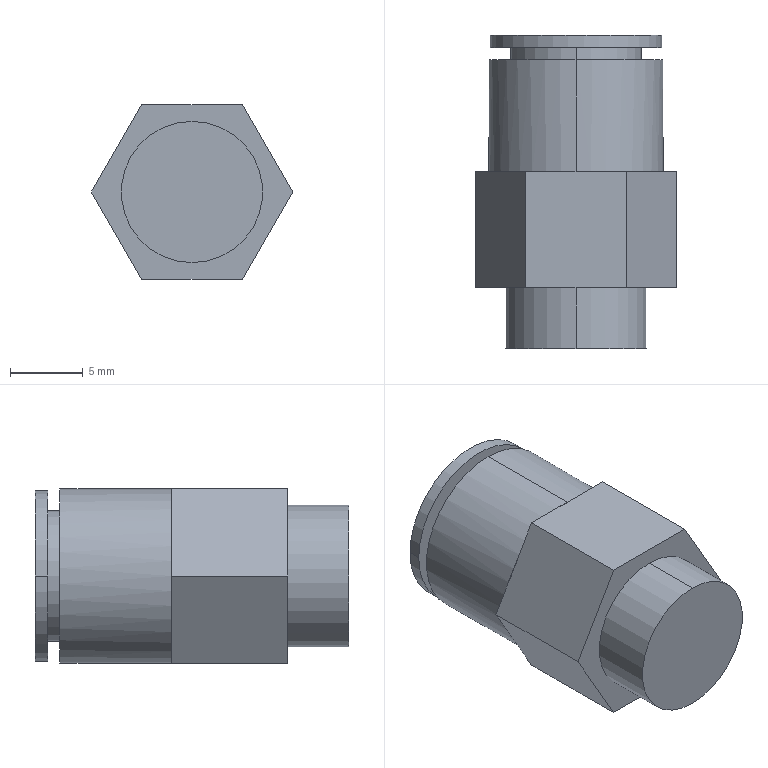Part | SolidWorks | features BaseBody 1 | 1 solid | 28 faces | box 13.856 x 21.6 x 12 mm | volume 1847 mm3 | plane 18 | cylinder 10 | commonest cylinder face diameters 6 x2 9 x2 9.728 x2 11.8 x2 12 x2
STEP:
#1=CARTESIAN_POINT('',(0.,1.5,3.));
#2=VERTEX_POINT('',#1);
#3=CARTESIAN_POINT('',(0.,1.5,-3.));
#4=VERTEX_POINT('',#3);
#5=CARTESIAN_POINT('',(0.,1.5,0.));
#6=DIRECTION('',(0.,-1.,0.));
#7=DIRECTION('',(0.,0.,1.));
#8=AXIS2_PLACEMENT_3D('',#5,#6,#7);
#9=CIRCLE('',#8,3.);
#10=EDGE_CURVE('',#2,#4,#9,.T.);
#11=ORIENTED_EDGE('',*,*,#10,.T.);
#12=CARTESIAN_POINT('',(0.,18.5,-3.));
#13=VERTEX_POINT('',#12);
#14=CARTESIAN_POINT('',(0.,1.5,-3.));
#15=DIRECTION('',(0.,1.,0.));
#16=VECTOR('',#15,1000.);
#17=LINE('',#14,#16);
#18=EDGE_CURVE('',#4,#13,#17,.T.);
#19=ORIENTED_EDGE('',*,*,#18,.T.);
#20=CARTESIAN_POINT('',(0.,18.5,3.));
#21=VERTEX_POINT('',#20);
#22=CARTESIAN_POINT('',(0.,18.5,0.));
#23=DIRECTION('',(0.,1.,0.));
#24=DIRECTION('',(0.,0.,1.));
#25=AXIS2_PLACEMENT_3D('',#22,#23,#24);
#26=CIRCLE('',#25,3.);
#27=EDGE_CURVE('',#13,#21,#26,.T.);
#28=ORIENTED_EDGE('',*,*,#27,.T.);
#29=CARTESIAN_POINT('',(0.,1.5,3.));
#30=DIRECTION('',(0.,1.,0.));
#31=VECTOR('',#30,1000.);
#32=LINE('',#29,#31);
#33=EDGE_CURVE('',#2,#21,#32,.T.);
#34=ORIENTED_EDGE('',*,*,#33,.F.);
#35=EDGE_LOOP('',(#11,#19,#28,#34));
#36=FACE_OUTER_BOUND('',#35,.T.);
#37=CARTESIAN_POINT('',(0.,1.5,0.));
#38=DIRECTION('',(0.,1.,0.));
#39=DIRECTION('',(0.,0.,1.));
#40=AXIS2_PLACEMENT_3D('',#37,#38,#39);
#41=CYLINDRICAL_SURFACE('',#40,3.);
#42=ADVANCED_FACE('',(#36),#41,.F.);
#43=CARTESIAN_POINT('',(-5.9,17.65,0.));
#44=VERTEX_POINT('',#43);
#45=CARTESIAN_POINT('',(5.9,17.65,0.));
#46=VERTEX_POINT('',#45);
#47=CARTESIAN_POINT('',(0.,17.65,0.));
#48=DIRECTION('',(0.,1.,0.));
#49=DIRECTION('',(-1.,0.,0.));
#50=AXIS2_PLACEMENT_3D('',#47,#48,#49);
#51=CIRCLE('',#50,5.9);
#52=EDGE_CURVE('',#44,#46,#51,.T.);
#53=ORIENTED_EDGE('',*,*,#52,.T.);
#54=CARTESIAN_POINT('',(5.9,18.5,0.));
#55=VERTEX_POINT('',#54);
#56=CARTESIAN_POINT('',(5.9,18.5,0.));
#57=DIRECTION('',(0.,1.,0.));
#58=VECTOR('',#57,1000.);
#59=LINE('',#56,#58);
#60=EDGE_CURVE('',#46,#55,#59,.T.);
#61=ORIENTED_EDGE('',*,*,#60,.T.);
#62=CARTESIAN_POINT('',(-5.9,18.5,0.));
#63=VERTEX_POINT('',#62);
#64=CARTESIAN_POINT('',(0.,18.5,0.));
#65=DIRECTION('',(0.,1.,0.));
#66=DIRECTION('',(-1.,0.,0.));
#67=AXIS2_PLACEMENT_3D('',#64,#65,#66);
#68=CIRCLE('',#67,5.9);
#69=EDGE_CURVE('',#63,#55,#68,.T.);
#70=ORIENTED_EDGE('',*,*,#69,.F.);
#71=CARTESIAN_POINT('',(-5.9,18.5,0.));
#72=DIRECTION('',(0.,1.,0.));
#73=VECTOR('',#72,1000.);
#74=LINE('',#71,#73);
#75=EDGE_CURVE('',#44,#63,#74,.T.);
#76=ORIENTED_EDGE('',*,*,#75,.F.);
#77=EDGE_LOOP('',(#53,#61,#70,#76));
#78=FACE_OUTER_BOUND('',#77,.T.);
#79=CARTESIAN_POINT('',(0.,18.5,0.));
#80=DIRECTION('',(0.,1.,0.));
#81=DIRECTION('',(-1.,0.,0.));
#82=AXIS2_PLACEMENT_3D('',#79,#80,#81);
#83=CYLINDRICAL_SURFACE('',#82,5.9);
#84=ADVANCED_FACE('',(#78),#83,.T.);
#85=CARTESIAN_POINT('',(0.,16.8,4.5));
#86=VERTEX_POINT('',#85);
#87=CARTESIAN_POINT('',(0.,16.8,-4.5));
#88=VERTEX_POINT('',#87);
#89=CARTESIAN_POINT('',(0.,16.8,0.));
#90=DIRECTION('',(0.,1.,0.));
#91=DIRECTION('',(0.,0.,1.));
#92=AXIS2_PLACEMENT_3D('',#89,#90,#91);
#93=CIRCLE('',#92,4.5);
#94=EDGE_CURVE('',#86,#88,#93,.T.);
#95=ORIENTED_EDGE('',*,*,#94,.T.);
#96=CARTESIAN_POINT('',(0.,17.65,-4.5));
#97=VERTEX_POINT('',#96);
#98=CARTESIAN_POINT('',(0.,17.65,-4.5));
#99=DIRECTION('',(0.,1.,0.));
#100=VECTOR('',#99,1000.);
#101=LINE('',#98,#100);
#102=EDGE_CURVE('',#88,#97,#101,.T.);
#103=ORIENTED_EDGE('',*,*,#102,.T.);
#104=CARTESIAN_POINT('',(0.,17.65,4.5));
#105=VERTEX_POINT('',#104);
#106=CARTESIAN_POINT('',(0.,17.65,0.));
#107=DIRECTION('',(0.,1.,0.));
#108=DIRECTION('',(0.,0.,1.));
#109=AXIS2_PLACEMENT_3D('',#106,#107,#108);
#110=CIRCLE('',#109,4.5);
#111=EDGE_CURVE('',#105,#97,#110,.T.);
#112=ORIENTED_EDGE('',*,*,#111,.F.);
#113=CARTESIAN_POINT('',(0.,17.65,4.5));
#114=DIRECTION('',(0.,1.,0.));
#115=VECTOR('',#114,1000.);
#116=LINE('',#113,#115);
#117=EDGE_CURVE('',#86,#105,#116,.T.);
#118=ORIENTED_EDGE('',*,*,#117,.F.);
#119=EDGE_LOOP('',(#95,#103,#112,#118));
#120=FACE_OUTER_BOUND('',#119,.T.);
#121=CARTESIAN_POINT('',(0.,17.65,0.));
#122=DIRECTION('',(0.,1.,0.));
#123=DIRECTION('',(0.,0.,1.));
#124=AXIS2_PLACEMENT_3D('',#121,#122,#123);
#125=CYLINDRICAL_SURFACE('',#124,4.5);
#126=ADVANCED_FACE('',(#120),#125,.T.);
#127=CARTESIAN_POINT('',(5.195,9.1,-3.001));
#128=VERTEX_POINT('',#127);
#129=CARTESIAN_POINT('',(0.,9.1,-6.));
#130=VERTEX_POINT('',#129);
#131=CARTESIAN_POINT('',(0.,9.1,0.));
#132=DIRECTION('',(0.,1.,0.));
#133=DIRECTION('',(0.,0.,1.));
#134=AXIS2_PLACEMENT_3D('',#131,#132,#133);
#135=CIRCLE('',#134,6.);
#136=EDGE_CURVE('',#128,#130,#135,.T.);
#137=ORIENTED_EDGE('',*,*,#136,.T.);
#138=CARTESIAN_POINT('',(0.,16.8,-6.));
#139=VERTEX_POINT('',#138);
#140=CARTESIAN_POINT('',(0.,16.8,-6.));
#141=DIRECTION('',(0.,1.,0.));
#142=VECTOR('',#141,1000.);
#143=LINE('',#140,#142);
#144=EDGE_CURVE('',#130,#139,#143,.T.);
#145=ORIENTED_EDGE('',*,*,#144,.T.);
#146=CARTESIAN_POINT('',(0.,16.8,6.));
#147=VERTEX_POINT('',#146);
#148=CARTESIAN_POINT('',(0.,16.8,0.));
#149=DIRECTION('',(0.,1.,0.));
#150=DIRECTION('',(0.,0.,1.));
#151=AXIS2_PLACEMENT_3D('',#148,#149,#150);
#152=CIRCLE('',#151,6.);
#153=EDGE_CURVE('',#147,#139,#152,.T.);
#154=ORIENTED_EDGE('',*,*,#153,.F.);
#155=CARTESIAN_POINT('',(0.,9.1,6.));
#156=VERTEX_POINT('',#155);
#157=CARTESIAN_POINT('',(0.,16.8,6.));
#158=DIRECTION('',(0.,1.,0.));
#159=VECTOR('',#158,1000.);
#160=LINE('',#157,#159);
#161=EDGE_CURVE('',#156,#147,#160,.T.);
#162=ORIENTED_EDGE('',*,*,#161,.F.);
#163=CARTESIAN_POINT('',(5.195,9.1,3.001));
#164=VERTEX_POINT('',#163);
#165=CARTESIAN_POINT('',(0.,9.1,0.));
#166=DIRECTION('',(0.,1.,0.));
#167=DIRECTION('',(0.,0.,1.));
#168=AXIS2_PLACEMENT_3D('',#165,#166,#167);
#169=CIRCLE('',#168,6.);
#170=EDGE_CURVE('',#156,#164,#169,.T.);
#171=ORIENTED_EDGE('',*,*,#170,.T.);
#172=CARTESIAN_POINT('',(5.197,9.1,2.999));
#173=VERTEX_POINT('',#172);
#174=CARTESIAN_POINT('',(5.196,9.1,3.));
#175=DIRECTION('',(-0.5,0.,0.866));
#176=VECTOR('',#175,1000.);
#177=LINE('',#174,#176);
#178=EDGE_CURVE('',#173,#164,#177,.T.);
#179=ORIENTED_EDGE('',*,*,#178,.F.);
#180=CARTESIAN_POINT('',(5.197,9.1,-2.999));
#181=VERTEX_POINT('',#180);
#182=CARTESIAN_POINT('',(0.,9.1,0.));
#183=DIRECTION('',(0.,1.,0.));
#184=DIRECTION('',(0.,0.,1.));
#185=AXIS2_PLACEMENT_3D('',#182,#183,#184);
#186=CIRCLE('',#185,6.);
#187=EDGE_CURVE('',#173,#181,#186,.T.);
#188=ORIENTED_EDGE('',*,*,#187,.T.);
#189=CARTESIAN_POINT('',(5.196,9.1,-3.));
#190=DIRECTION('',(0.5,0.,0.866));
#191=VECTOR('',#190,1000.);
#192=LINE('',#189,#191);
#193=EDGE_CURVE('',#128,#181,#192,.T.);
#194=ORIENTED_EDGE('',*,*,#193,.F.);
#195=EDGE_LOOP('',(#137,#145,#154,#162,#171,#179,#188,#194));
#196=FACE_OUTER_BOUND('',#195,.T.);
#197=CARTESIAN_POINT('',(0.,16.8,0.));
#198=DIRECTION('',(0.,1.,0.));
#199=DIRECTION('',(0.,0.,1.));
#200=AXIS2_PLACEMENT_3D('',#197,#198,#199);
#201=CYLINDRICAL_SURFACE('',#200,6.);
#202=ADVANCED_FACE('',(#196),#201,.T.);
#203=CARTESIAN_POINT('',(0.,-3.1,4.864));
#204=VERTEX_POINT('',#203);
#205=CARTESIAN_POINT('',(0.,-3.1,-4.864));
#206=VERTEX_POINT('',#205);
#207=CARTESIAN_POINT('',(0.,-3.1,0.));
#208=DIRECTION('',(0.,1.,0.));
#209=DIRECTION('',(0.,0.,1.));
#210=AXIS2_PLACEMENT_3D('',#207,#208,#209);
#211=CIRCLE('',#210,4.864);
#212=EDGE_CURVE('',#204,#206,#211,.T.);
#213=ORIENTED_EDGE('',*,*,#212,.T.);
#214=CARTESIAN_POINT('',(0.,1.1,-4.864));
#215=VERTEX_POINT('',#214);
#216=CARTESIAN_POINT('',(0.,1.1,-4.864));
#217=DIRECTION('',(0.,1.,0.));
#218=VECTOR('',#217,1000.);
#219=LINE('',#216,#218);
#220=EDGE_CURVE('',#206,#215,#219,.T.);
#221=ORIENTED_EDGE('',*,*,#220,.T.);
#222=CARTESIAN_POINT('',(0.,1.1,4.864));
#223=VERTEX_POINT('',#222);
#224=CARTESIAN_POINT('',(0.,1.1,0.));
#225=DIRECTION('',(0.,1.,0.));
#226=DIRECTION('',(0.,0.,1.));
#227=AXIS2_PLACEMENT_3D('',#224,#225,#226);
#228=CIRCLE('',#227,4.864);
#229=EDGE_CURVE('',#223,#215,#228,.T.);
#230=ORIENTED_EDGE('',*,*,#229,.F.);
#231=CARTESIAN_POINT('',(0.,1.1,4.864));
#232=DIRECTION('',(0.,1.,0.));
#233=VECTOR('',#232,1000.);
#234=LINE('',#231,#233);
#235=EDGE_CURVE('',#204,#223,#234,.T.);
#236=ORIENTED_EDGE('',*,*,#235,.F.);
#237=EDGE_LOOP('',(#213,#221,#230,#236));
#238=FACE_OUTER_BOUND('',#237,.T.);
#239=CARTESIAN_POINT('',(0.,1.1,0.));
#240=DIRECTION('',(0.,1.,0.));
#241=DIRECTION('',(0.,0.,1.));
#242=AXIS2_PLACEMENT_3D('',#239,#240,#241);
#243=CYLINDRICAL_SURFACE('',#242,4.864);
#244=ADVANCED_FACE('',(#238),#243,.T.);
#245=ORIENTED_EDGE('',*,*,#18,.F.);
#246=CARTESIAN_POINT('',(0.,1.5,0.));
#247=DIRECTION('',(0.,-1.,0.));
#248=DIRECTION('',(0.,0.,1.));
#249=AXIS2_PLACEMENT_3D('',#246,#247,#248);
#250=CIRCLE('',#249,3.);
#251=EDGE_CURVE('',#4,#2,#250,.T.);
#252=ORIENTED_EDGE('',*,*,#251,.T.);
#253=ORIENTED_EDGE('',*,*,#33,.T.);
#254=CARTESIAN_POINT('',(0.,18.5,0.));
#255=DIRECTION('',(0.,1.,0.));
#256=DIRECTION('',(0.,0.,1.));
#257=AXIS2_PLACEMENT_3D('',#254,#255,#256);
#258=CIRCLE('',#257,3.);
#259=EDGE_CURVE('',#21,#13,#258,.T.);
#260=ORIENTED_EDGE('',*,*,#259,.T.);
#261=EDGE_LOOP('',(#245,#252,#253,#260));
#262=FACE_OUTER_BOUND('',#261,.T.);
#263=CARTESIAN_POINT('',(0.,1.5,0.));
#264=DIRECTION('',(0.,1.,0.));
#265=DIRECTION('',(0.,0.,1.));
#266=AXIS2_PLACEMENT_3D('',#263,#264,#265);
#267=CYLINDRICAL_SURFACE('',#266,3.);
#268=ADVANCED_FACE('',(#262),#267,.F.);
#269=ORIENTED_EDGE('',*,*,#259,.F.);
#270=ORIENTED_EDGE('',*,*,#27,.F.);
#271=EDGE_LOOP('',(#269,#270));
#272=FACE_BOUND('',#271,.T.);
#273=ORIENTED_EDGE('',*,*,#69,.T.);
#274=CARTESIAN_POINT('',(0.,18.5,0.));
#275=DIRECTION('',(0.,1.,0.));
#276=DIRECTION('',(-1.,0.,0.));
#277=AXIS2_PLACEMENT_3D('',#274,#275,#276);
#278=CIRCLE('',#277,5.9);
#279=EDGE_CURVE('',#55,#63,#278,.T.);
#280=ORIENTED_EDGE('',*,*,#279,.T.);
#281=EDGE_LOOP('',(#273,#280));
#282=FACE_OUTER_BOUND('',#281,.T.);
#283=CARTESIAN_POINT('',(5.971,18.5,5.9));
#284=DIRECTION('',(0.,1.,0.));
#285=DIRECTION('',(0.,0.,-1.));
#286=AXIS2_PLACEMENT_3D('',#283,#284,#285);
#287=PLANE('',#286);
#288=ADVANCED_FACE('',(#272,#282),#287,.T.);
#289=ORIENTED_EDGE('',*,*,#10,.F.);
#290=ORIENTED_EDGE('',*,*,#251,.F.);
#291=EDGE_LOOP('',(#289,#290));
#292=FACE_OUTER_BOUND('',#291,.T.);
#293=CARTESIAN_POINT('',(3.036,1.5,3.));
#294=DIRECTION('',(0.,1.,0.));
#295=DIRECTION('',(0.,0.,-1.));
#296=AXIS2_PLACEMENT_3D('',#293,#294,#295);
#297=PLANE('',#296);
#298=ADVANCED_FACE('',(#292),#297,.T.);
#299=ORIENTED_EDGE('',*,*,#60,.F.);
#300=CARTESIAN_POINT('',(0.,17.65,0.));
#301=DIRECTION('',(0.,1.,0.));
#302=DIRECTION('',(-1.,0.,0.));
#303=AXIS2_PLACEMENT_3D('',#300,#301,#302);
#304=CIRCLE('',#303,5.9);
#305=EDGE_CURVE('',#46,#44,#304,.T.);
#306=ORIENTED_EDGE('',*,*,#305,.T.);
#307=ORIENTED_EDGE('',*,*,#75,.T.);
#308=ORIENTED_EDGE('',*,*,#279,.F.);
#309=EDGE_LOOP('',(#299,#306,#307,#308));
#310=FACE_OUTER_BOUND('',#309,.T.);
#311=CARTESIAN_POINT('',(0.,18.5,0.));
#312=DIRECTION('',(0.,1.,0.));
#313=DIRECTION('',(-1.,0.,0.));
#314=AXIS2_PLACEMENT_3D('',#311,#312,#313);
#315=CYLINDRICAL_SURFACE('',#314,5.9);
#316=ADVANCED_FACE('',(#310),#315,.T.);
#317=ORIENTED_EDGE('',*,*,#111,.T.);
#318=CARTESIAN_POINT('',(0.,17.65,0.));
#319=DIRECTION('',(0.,1.,0.));
#320=DIRECTION('',(0.,0.,1.));
#321=AXIS2_PLACEMENT_3D('',#318,#319,#320);
#322=CIRCLE('',#321,4.5);
#323=EDGE_CURVE('',#97,#105,#322,.T.);
#324=ORIENTED_EDGE('',*,*,#323,.T.);
#325=EDGE_LOOP('',(#317,#324));
#326=FACE_BOUND('',#325,.T.);
#327=ORIENTED_EDGE('',*,*,#52,.F.);
#328=ORIENTED_EDGE('',*,*,#305,.F.);
#329=EDGE_LOOP('',(#327,#328));
#330=FACE_OUTER_BOUND('',#329,.T.);
#331=CARTESIAN_POINT('',(5.971,17.65,-5.9));
#332=DIRECTION('',(0.,-1.,0.));
#333=DIRECTION('',(0.,0.,1.));
#334=AXIS2_PLACEMENT_3D('',#331,#332,#333);
#335=PLANE('',#334);
#336=ADVANCED_FACE('',(#326,#330),#335,.T.);
#337=ORIENTED_EDGE('',*,*,#102,.F.);
#338=CARTESIAN_POINT('',(0.,16.8,0.));
#339=DIRECTION('',(0.,1.,0.));
#340=DIRECTION('',(0.,0.,1.));
#341=AXIS2_PLACEMENT_3D('',#338,#339,#340);
#342=CIRCLE('',#341,4.5);
#343=EDGE_CURVE('',#88,#86,#342,.T.);
#344=ORIENTED_EDGE('',*,*,#343,.T.);
#345=ORIENTED_EDGE('',*,*,#117,.T.);
#346=ORIENTED_EDGE('',*,*,#323,.F.);
#347=EDGE_LOOP('',(#337,#344,#345,#346));
#348=FACE_OUTER_BOUND('',#347,.T.);
#349=CARTESIAN_POINT('',(0.,17.65,0.));
#350=DIRECTION('',(0.,1.,0.));
#351=DIRECTION('',(0.,0.,1.));
#352=AXIS2_PLACEMENT_3D('',#349,#350,#351);
#353=CYLINDRICAL_SURFACE('',#352,4.5);
#354=ADVANCED_FACE('',(#348),#353,.T.);
#355=ORIENTED_EDGE('',*,*,#94,.F.);
#356=ORIENTED_EDGE('',*,*,#343,.F.);
#357=EDGE_LOOP('',(#355,#356));
#358=FACE_BOUND('',#357,.T.);
#359=ORIENTED_EDGE('',*,*,#153,.T.);
#360=CARTESIAN_POINT('',(0.,16.8,0.));
#361=DIRECTION('',(0.,1.,0.));
#362=DIRECTION('',(0.,0.,1.));
#363=AXIS2_PLACEMENT_3D('',#360,#361,#362);
#364=CIRCLE('',#363,6.);
#365=EDGE_CURVE('',#139,#147,#364,.T.);
#366=ORIENTED_EDGE('',*,*,#365,.T.);
#367=EDGE_LOOP('',(#359,#366));
#368=FACE_OUTER_BOUND('',#367,.T.);
#369=CARTESIAN_POINT('',(6.072,16.8,6.));
#370=DIRECTION('',(0.,1.,0.));
#371=DIRECTION('',(0.,0.,-1.));
#372=AXIS2_PLACEMENT_3D('',#369,#370,#371);
#373=PLANE('',#372);
#374=ADVANCED_FACE('',(#358,#368),#373,.T.);
#375=ORIENTED_EDGE('',*,*,#144,.F.);
#376=CARTESIAN_POINT('',(-5.195,9.1,-3.001));
#377=VERTEX_POINT('',#376);
#378=CARTESIAN_POINT('',(0.,9.1,0.));
#379=DIRECTION('',(0.,1.,0.));
#380=DIRECTION('',(0.,0.,1.));
#381=AXIS2_PLACEMENT_3D('',#378,#379,#380);
#382=CIRCLE('',#381,6.);
#383=EDGE_CURVE('',#130,#377,#382,.T.);
#384=ORIENTED_EDGE('',*,*,#383,.T.);
#385=CARTESIAN_POINT('',(-5.197,9.1,-2.999));
#386=VERTEX_POINT('',#385);
#387=CARTESIAN_POINT('',(-5.196,9.1,-3.));
#388=DIRECTION('',(0.5,0.,-0.866));
#389=VECTOR('',#388,1000.);
#390=LINE('',#387,#389);
#391=EDGE_CURVE('',#386,#377,#390,.T.);
#392=ORIENTED_EDGE('',*,*,#391,.F.);
#393=CARTESIAN_POINT('',(-5.197,9.1,2.999));
#394=VERTEX_POINT('',#393);
#395=CARTESIAN_POINT('',(0.,9.1,0.));
#396=DIRECTION('',(0.,1.,0.));
#397=DIRECTION('',(0.,0.,1.));
#398=AXIS2_PLACEMENT_3D('',#395,#396,#397);
#399=CIRCLE('',#398,6.);
#400=EDGE_CURVE('',#386,#394,#399,.T.);
#401=ORIENTED_EDGE('',*,*,#400,.T.);
#402=CARTESIAN_POINT('',(-5.195,9.1,3.001));
#403=VERTEX_POINT('',#402);
#404=CARTESIAN_POINT('',(-5.196,9.1,3.));
#405=DIRECTION('',(-0.5,0.,-0.866));
#406=VECTOR('',#405,1000.);
#407=LINE('',#404,#406);
#408=EDGE_CURVE('',#403,#394,#407,.T.);
#409=ORIENTED_EDGE('',*,*,#408,.F.);
#410=CARTESIAN_POINT('',(0.,9.1,0.));
#411=DIRECTION('',(0.,1.,0.));
#412=DIRECTION('',(0.,0.,1.));
#413=AXIS2_PLACEMENT_3D('',#410,#411,#412);
#414=CIRCLE('',#413,6.);
#415=EDGE_CURVE('',#403,#156,#414,.T.);
#416=ORIENTED_EDGE('',*,*,#415,.T.);
#417=ORIENTED_EDGE('',*,*,#161,.T.);
#418=ORIENTED_EDGE('',*,*,#365,.F.);
#419=EDGE_LOOP('',(#375,#384,#392,#401,#409,#416,#417,#418));
#420=FACE_OUTER_BOUND('',#419,.T.);
#421=CARTESIAN_POINT('',(0.,16.8,0.));
#422=DIRECTION('',(0.,1.,0.));
#423=DIRECTION('',(0.,0.,1.));
#424=AXIS2_PLACEMENT_3D('',#421,#422,#423);
#425=CYLINDRICAL_SURFACE('',#424,6.);
#426=ADVANCED_FACE('',(#420),#425,.T.);
#427=CARTESIAN_POINT('',(3.464,9.1,-6.));
#428=VERTEX_POINT('',#427);
#429=CARTESIAN_POINT('',(5.195,9.1,-3.001));
#430=CARTESIAN_POINT('',(4.618,9.1,-4.001));
#431=CARTESIAN_POINT('',(4.041,9.1,-5.));
#432=CARTESIAN_POINT('',(3.464,9.1,-6.));
#433=B_SPLINE_CURVE_WITH_KNOTS('',3,(#429,#430,#431,#432),.UNSPECIFIED.,.F.,.F.,(4,4),(0.0004567,1.),.UNSPECIFIED.);
#434=EDGE_CURVE('',#128,#428,#433,.T.);
#435=ORIENTED_EDGE('',*,*,#434,.T.);
#436=CARTESIAN_POINT('',(0.,9.1,-6.));
#437=DIRECTION('',(-1.,0.,0.));
#438=VECTOR('',#437,1000.);
#439=LINE('',#436,#438);
#440=EDGE_CURVE('',#428,#130,#439,.T.);
#441=ORIENTED_EDGE('',*,*,#440,.T.);
#442=ORIENTED_EDGE('',*,*,#136,.F.);
#443=EDGE_LOOP('',(#435,#441,#442));
#444=FACE_OUTER_BOUND('',#443,.T.);
#445=CARTESIAN_POINT('',(-0.03117,9.1,-6.));
#446=DIRECTION('',(0.,1.,0.));
#447=DIRECTION('',(0.,0.,1.));
#448=AXIS2_PLACEMENT_3D('',#445,#446,#447);
#449=PLANE('',#448);
#450=ADVANCED_FACE('',(#444),#449,.T.);
#451=CARTESIAN_POINT('',(6.928,9.1,0.000000144));
#452=VERTEX_POINT('',#451);
#453=CARTESIAN_POINT('',(5.197,9.1,2.999));
#454=CARTESIAN_POINT('',(5.774,9.1,1.999));
#455=CARTESIAN_POINT('',(6.351,9.1,0.9995));
#456=CARTESIAN_POINT('',(6.928,9.1,0.000000144));
#457=B_SPLINE_CURVE_WITH_KNOTS('',3,(#453,#454,#455,#456),.UNSPECIFIED.,.F.,.F.,(4,4),(0.0004567,1.),.UNSPECIFIED.);
#458=EDGE_CURVE('',#173,#452,#457,.T.);
#459=ORIENTED_EDGE('',*,*,#458,.T.);
#460=CARTESIAN_POINT('',(6.928,9.1,0.000000144));
#461=CARTESIAN_POINT('',(6.351,9.1,-0.9995));
#462=CARTESIAN_POINT('',(5.774,9.1,-1.999));
#463=CARTESIAN_POINT('',(5.197,9.1,-2.999));
#464=B_SPLINE_CURVE_WITH_KNOTS('',3,(#460,#461,#462,#463),.UNSPECIFIED.,.F.,.F.,(4,4),(0.,0.9995),.UNSPECIFIED.);
#465=EDGE_CURVE('',#452,#181,#464,.T.);
#466=ORIENTED_EDGE('',*,*,#465,.T.);
#467=ORIENTED_EDGE('',*,*,#187,.F.);
#468=EDGE_LOOP('',(#459,#466,#467));
#469=FACE_OUTER_BOUND('',#468,.T.);
#470=CARTESIAN_POINT('',(5.187,9.1,-3.));
#471=DIRECTION('',(0.,1.,0.));
#472=DIRECTION('',(0.,0.,1.));
#473=AXIS2_PLACEMENT_3D('',#470,#471,#472);
#474=PLANE('',#473);
#475=ADVANCED_FACE('',(#469),#474,.T.);
#476=CARTESIAN_POINT('',(3.464,9.1,6.));
#477=VERTEX_POINT('',#476);
#478=CARTESIAN_POINT('',(0.,9.1,6.));
#479=DIRECTION('',(1.,0.,0.));
#480=VECTOR('',#479,1000.);
#481=LINE('',#478,#480);
#482=EDGE_CURVE('',#156,#477,#481,.T.);
#483=ORIENTED_EDGE('',*,*,#482,.T.);
#484=CARTESIAN_POINT('',(3.464,9.1,6.));
#485=CARTESIAN_POINT('',(4.041,9.1,5.));
#486=CARTESIAN_POINT('',(4.618,9.1,4.001));
#487=CARTESIAN_POINT('',(5.195,9.1,3.001));
#488=B_SPLINE_CURVE_WITH_KNOTS('',3,(#484,#485,#486,#487),.UNSPECIFIED.,.F.,.F.,(4,4),(0.,0.9995),.UNSPECIFIED.);
#489=EDGE_CURVE('',#477,#164,#488,.T.);
#490=ORIENTED_EDGE('',*,*,#489,.T.);
#491=ORIENTED_EDGE('',*,*,#170,.F.);
#492=EDGE_LOOP('',(#483,#490,#491));
#493=FACE_OUTER_BOUND('',#492,.T.);
#494=CARTESIAN_POINT('',(-0.03117,9.1,3.));
#495=DIRECTION('',(0.,1.,0.));
#496=DIRECTION('',(0.,0.,1.));
#497=AXIS2_PLACEMENT_3D('',#494,#495,#496);
#498=PLANE('',#497);
#499=ADVANCED_FACE('',(#493),#498,.T.);
#500=CARTESIAN_POINT('',(-3.464,9.1,6.));
#501=VERTEX_POINT('',#500);
#502=CARTESIAN_POINT('',(-5.195,9.1,3.001));
#503=CARTESIAN_POINT('',(-4.618,9.1,4.001));
#504=CARTESIAN_POINT('',(-4.041,9.1,5.));
#505=CARTESIAN_POINT('',(-3.464,9.1,6.));
#506=B_SPLINE_CURVE_WITH_KNOTS('',3,(#502,#503,#504,#505),.UNSPECIFIED.,.F.,.F.,(4,4),(0.0004567,1.),.UNSPECIFIED.);
#507=EDGE_CURVE('',#403,#501,#506,.T.);
#508=ORIENTED_EDGE('',*,*,#507,.T.);
#509=CARTESIAN_POINT('',(-5.196,9.1,6.));
#510=DIRECTION('',(1.,0.,0.));
#511=VECTOR('',#510,1000.);
#512=LINE('',#509,#511);
#513=EDGE_CURVE('',#501,#156,#512,.T.);
#514=ORIENTED_EDGE('',*,*,#513,.T.);
#515=ORIENTED_EDGE('',*,*,#415,.F.);
#516=EDGE_LOOP('',(#508,#514,#515));
#517=FACE_OUTER_BOUND('',#516,.T.);
#518=CARTESIAN_POINT('',(-5.227,9.1,3.));
#519=DIRECTION('',(0.,1.,0.));
#520=DIRECTION('',(0.,0.,1.));
#521=AXIS2_PLACEMENT_3D('',#518,#519,#520);
#522=PLANE('',#521);
#523=ADVANCED_FACE('',(#517),#522,.T.);
#524=CARTESIAN_POINT('',(-6.928,9.1,-0.000000144));
#525=VERTEX_POINT('',#524);
#526=CARTESIAN_POINT('',(-5.197,9.1,-2.999));
#527=CARTESIAN_POINT('',(-5.774,9.1,-1.999));
#528=CARTESIAN_POINT('',(-6.351,9.1,-0.9995));
#529=CARTESIAN_POINT('',(-6.928,9.1,-0.000000144));
#530=B_SPLINE_CURVE_WITH_KNOTS('',3,(#526,#527,#528,#529),.UNSPECIFIED.,.F.,.F.,(4,4),(0.0004567,1.),.UNSPECIFIED.);
#531=EDGE_CURVE('',#386,#525,#530,.T.);
#532=ORIENTED_EDGE('',*,*,#531,.T.);
#533=CARTESIAN_POINT('',(-6.928,9.1,-0.000000144));
#534=CARTESIAN_POINT('',(-6.351,9.1,0.9995));
#535=CARTESIAN_POINT('',(-5.774,9.1,1.999));
#536=CARTESIAN_POINT('',(-5.197,9.1,2.999));
#537=B_SPLINE_CURVE_WITH_KNOTS('',3,(#533,#534,#535,#536),.UNSPECIFIED.,.F.,.F.,(4,4),(0.,0.9995),.UNSPECIFIED.);
#538=EDGE_CURVE('',#525,#394,#537,.T.);
#539=ORIENTED_EDGE('',*,*,#538,.T.);
#540=ORIENTED_EDGE('',*,*,#400,.F.);
#541=EDGE_LOOP('',(#532,#539,#540));
#542=FACE_OUTER_BOUND('',#541,.T.);
#543=CARTESIAN_POINT('',(-6.939,9.1,-3.));
#544=DIRECTION('',(0.,1.,0.));
#545=DIRECTION('',(0.,0.,1.));
#546=AXIS2_PLACEMENT_3D('',#543,#544,#545);
#547=PLANE('',#546);
#548=ADVANCED_FACE('',(#542),#547,.T.);
#549=CARTESIAN_POINT('',(-3.464,9.1,-6.));
#550=VERTEX_POINT('',#549);
#551=CARTESIAN_POINT('',(-5.196,9.1,-6.));
#552=DIRECTION('',(-1.,0.,0.));
#553=VECTOR('',#552,1000.);
#554=LINE('',#551,#553);
#555=EDGE_CURVE('',#130,#550,#554,.T.);
#556=ORIENTED_EDGE('',*,*,#555,.T.);
#557=CARTESIAN_POINT('',(-3.464,9.1,-6.));
#558=CARTESIAN_POINT('',(-4.041,9.1,-5.));
#559=CARTESIAN_POINT('',(-4.618,9.1,-4.001));
#560=CARTESIAN_POINT('',(-5.195,9.1,-3.001));
#561=B_SPLINE_CURVE_WITH_KNOTS('',3,(#557,#558,#559,#560),.UNSPECIFIED.,.F.,.F.,(4,4),(0.,0.9995),.UNSPECIFIED.);
#562=EDGE_CURVE('',#550,#377,#561,.T.);
#563=ORIENTED_EDGE('',*,*,#562,.T.);
#564=ORIENTED_EDGE('',*,*,#383,.F.);
#565=EDGE_LOOP('',(#556,#563,#564));
#566=FACE_OUTER_BOUND('',#565,.T.);
#567=CARTESIAN_POINT('',(-5.227,9.1,-6.));
#568=DIRECTION('',(0.,1.,0.));
#569=DIRECTION('',(0.,0.,1.));
#570=AXIS2_PLACEMENT_3D('',#567,#568,#569);
#571=PLANE('',#570);
#572=ADVANCED_FACE('',(#566),#571,.T.);
#573=ORIENTED_EDGE('',*,*,#440,.F.);
#574=CARTESIAN_POINT('',(3.464,1.1,-6.));
#575=VERTEX_POINT('',#574);
#576=CARTESIAN_POINT('',(3.464,9.1,-6.));
#577=DIRECTION('',(0.,-1.,0.));
#578=VECTOR('',#577,1000.);
#579=LINE('',#576,#578);
#580=EDGE_CURVE('',#428,#575,#579,.T.);
#581=ORIENTED_EDGE('',*,*,#580,.T.);
#582=CARTESIAN_POINT('',(-3.464,1.1,-6.));
#583=VERTEX_POINT('',#582);
#584=CARTESIAN_POINT('',(0.,1.1,-6.));
#585=DIRECTION('',(-1.,0.,0.));
#586=VECTOR('',#585,1000.);
#587=LINE('',#584,#586);
#588=EDGE_CURVE('',#575,#583,#587,.T.);
#589=ORIENTED_EDGE('',*,*,#588,.T.);
#590=CARTESIAN_POINT('',(-3.464,9.1,-6.));
#591=DIRECTION('',(0.,1.,0.));
#592=VECTOR('',#591,1000.);
#593=LINE('',#590,#592);
#594=EDGE_CURVE('',#583,#550,#593,.T.);
#595=ORIENTED_EDGE('',*,*,#594,.T.);
#596=ORIENTED_EDGE('',*,*,#555,.F.);
#597=EDGE_LOOP('',(#573,#581,#589,#595,#596));
#598=FACE_OUTER_BOUND('',#597,.T.);
#599=CARTESIAN_POINT('',(-3.464,9.1,-6.));
#600=DIRECTION('',(0.,0.,-1.));
#601=DIRECTION('',(1.,0.,0.));
#602=AXIS2_PLACEMENT_3D('',#599,#600,#601);
#603=PLANE('',#602);
#604=ADVANCED_FACE('',(#598),#603,.T.);
#605=ORIENTED_EDGE('',*,*,#193,.T.);
#606=ORIENTED_EDGE('',*,*,#465,.F.);
#607=CARTESIAN_POINT('',(6.928,1.1,0.));
#608=VERTEX_POINT('',#607);
#609=CARTESIAN_POINT('',(6.928,9.1,0.));
#610=DIRECTION('',(0.,-1.,0.));
#611=VECTOR('',#610,1000.);
#612=LINE('',#609,#611);
#613=EDGE_CURVE('',#452,#608,#612,.T.);
#614=ORIENTED_EDGE('',*,*,#613,.T.);
#615=CARTESIAN_POINT('',(5.196,1.1,-3.));
#616=DIRECTION('',(-0.5,0.,-0.866));
#617=VECTOR('',#616,1000.);
#618=LINE('',#615,#617);
#619=EDGE_CURVE('',#608,#575,#618,.T.);
#620=ORIENTED_EDGE('',*,*,#619,.T.);
#621=ORIENTED_EDGE('',*,*,#580,.F.);
#622=ORIENTED_EDGE('',*,*,#434,.F.);
#623=EDGE_LOOP('',(#605,#606,#614,#620,#621,#622));
#624=FACE_OUTER_BOUND('',#623,.T.);
#625=CARTESIAN_POINT('',(3.464,9.1,-6.));
#626=DIRECTION('',(0.866,0.,-0.5));
#627=DIRECTION('',(0.5,0.,0.866));
#628=AXIS2_PLACEMENT_3D('',#625,#626,#627);
#629=PLANE('',#628);
#630=ADVANCED_FACE('',(#624),#629,.T.);
#631=ORIENTED_EDGE('',*,*,#178,.T.);
#632=ORIENTED_EDGE('',*,*,#489,.F.);
#633=CARTESIAN_POINT('',(3.464,1.1,6.));
#634=VERTEX_POINT('',#633);
#635=CARTESIAN_POINT('',(3.464,9.1,6.));
#636=DIRECTION('',(0.,-1.,0.));
#637=VECTOR('',#636,1000.);
#638=LINE('',#635,#637);
#639=EDGE_CURVE('',#477,#634,#638,.T.);
#640=ORIENTED_EDGE('',*,*,#639,.T.);
#641=CARTESIAN_POINT('',(5.196,1.1,3.));
#642=DIRECTION('',(0.5,0.,-0.866));
#643=VECTOR('',#642,1000.);
#644=LINE('',#641,#643);
#645=EDGE_CURVE('',#634,#608,#644,.T.);
#646=ORIENTED_EDGE('',*,*,#645,.T.);
#647=ORIENTED_EDGE('',*,*,#613,.F.);
#648=ORIENTED_EDGE('',*,*,#458,.F.);
#649=EDGE_LOOP('',(#631,#632,#640,#646,#647,#648));
#650=FACE_OUTER_BOUND('',#649,.T.);
#651=CARTESIAN_POINT('',(6.928,9.1,0.));
#652=DIRECTION('',(0.866,0.,0.5));
#653=DIRECTION('',(-0.5,0.,0.866));
#654=AXIS2_PLACEMENT_3D('',#651,#652,#653);
#655=PLANE('',#654);
#656=ADVANCED_FACE('',(#650),#655,.T.);
#657=ORIENTED_EDGE('',*,*,#513,.F.);
#658=CARTESIAN_POINT('',(-3.464,1.1,6.));
#659=VERTEX_POINT('',#658);
#660=CARTESIAN_POINT('',(-3.464,9.1,6.));
#661=DIRECTION('',(0.,-1.,0.));
#662=VECTOR('',#661,1000.);
#663=LINE('',#660,#662);
#664=EDGE_CURVE('',#501,#659,#663,.T.);
#665=ORIENTED_EDGE('',*,*,#664,.T.);
#666=CARTESIAN_POINT('',(0.,1.1,6.));
#667=DIRECTION('',(1.,0.,0.));
#668=VECTOR('',#667,1000.);
#669=LINE('',#666,#668);
#670=EDGE_CURVE('',#659,#634,#669,.T.);
#671=ORIENTED_EDGE('',*,*,#670,.T.);
#672=ORIENTED_EDGE('',*,*,#639,.F.);
#673=ORIENTED_EDGE('',*,*,#482,.F.);
#674=EDGE_LOOP('',(#657,#665,#671,#672,#673));
#675=FACE_OUTER_BOUND('',#674,.T.);
#676=CARTESIAN_POINT('',(3.464,9.1,6.));
#677=DIRECTION('',(0.,0.,1.));
#678=DIRECTION('',(-1.,0.,0.));
#679=AXIS2_PLACEMENT_3D('',#676,#677,#678);
#680=PLANE('',#679);
#681=ADVANCED_FACE('',(#675),#680,.T.);
#682=ORIENTED_EDGE('',*,*,#408,.T.);
#683=ORIENTED_EDGE('',*,*,#538,.F.);
#684=CARTESIAN_POINT('',(-6.928,1.1,0.));
#685=VERTEX_POINT('',#684);
#686=CARTESIAN_POINT('',(-6.928,9.1,0.));
#687=DIRECTION('',(0.,-1.,0.));
#688=VECTOR('',#687,1000.);
#689=LINE('',#686,#688);
#690=EDGE_CURVE('',#525,#685,#689,.T.);
#691=ORIENTED_EDGE('',*,*,#690,.T.);
#692=CARTESIAN_POINT('',(-5.196,1.1,3.));
#693=DIRECTION('',(0.5,0.,0.866));
#694=VECTOR('',#693,1000.);
#695=LINE('',#692,#694);
#696=EDGE_CURVE('',#685,#659,#695,.T.);
#697=ORIENTED_EDGE('',*,*,#696,.T.);
#698=ORIENTED_EDGE('',*,*,#664,.F.);
#699=ORIENTED_EDGE('',*,*,#507,.F.);
#700=EDGE_LOOP('',(#682,#683,#691,#697,#698,#699));
#701=FACE_OUTER_BOUND('',#700,.T.);
#702=CARTESIAN_POINT('',(-3.464,9.1,6.));
#703=DIRECTION('',(-0.866,0.,0.5));
#704=DIRECTION('',(-0.5,0.,-0.866));
#705=AXIS2_PLACEMENT_3D('',#702,#703,#704);
#706=PLANE('',#705);
#707=ADVANCED_FACE('',(#701),#706,.T.);
#708=ORIENTED_EDGE('',*,*,#391,.T.);
#709=ORIENTED_EDGE('',*,*,#562,.F.);
#710=ORIENTED_EDGE('',*,*,#594,.F.);
#711=CARTESIAN_POINT('',(-5.196,1.1,-3.));
#712=DIRECTION('',(-0.5,0.,0.866));
#713=VECTOR('',#712,1000.);
#714=LINE('',#711,#713);
#715=EDGE_CURVE('',#583,#685,#714,.T.);
#716=ORIENTED_EDGE('',*,*,#715,.T.);
#717=ORIENTED_EDGE('',*,*,#690,.F.);
#718=ORIENTED_EDGE('',*,*,#531,.F.);
#719=EDGE_LOOP('',(#708,#709,#710,#716,#717,#718));
#720=FACE_OUTER_BOUND('',#719,.T.);
#721=CARTESIAN_POINT('',(-6.928,9.1,0.));
#722=DIRECTION('',(-0.866,0.,-0.5));
#723=DIRECTION('',(0.5,0.,-0.866));
#724=AXIS2_PLACEMENT_3D('',#721,#722,#723);
#725=PLANE('',#724);
#726=ADVANCED_FACE('',(#720),#725,.T.);
#727=ORIENTED_EDGE('',*,*,#229,.T.);
#728=CARTESIAN_POINT('',(0.,1.1,0.));
#729=DIRECTION('',(0.,1.,0.));
#730=DIRECTION('',(0.,0.,1.));
#731=AXIS2_PLACEMENT_3D('',#728,#729,#730);
#732=CIRCLE('',#731,4.864);
#733=EDGE_CURVE('',#215,#223,#732,.T.);
#734=ORIENTED_EDGE('',*,*,#733,.T.);
#735=EDGE_LOOP('',(#727,#734));
#736=FACE_BOUND('',#735,.T.);
#737=ORIENTED_EDGE('',*,*,#588,.F.);
#738=ORIENTED_EDGE('',*,*,#619,.F.);
#739=ORIENTED_EDGE('',*,*,#645,.F.);
#740=ORIENTED_EDGE('',*,*,#670,.F.);
#741=ORIENTED_EDGE('',*,*,#696,.F.);
#742=ORIENTED_EDGE('',*,*,#715,.F.);
#743=EDGE_LOOP('',(#737,#738,#739,#740,#741,#742));
#744=FACE_OUTER_BOUND('',#743,.T.);
#745=CARTESIAN_POINT('',(7.011,1.1,-6.));
#746=DIRECTION('',(0.,-1.,0.));
#747=DIRECTION('',(0.,0.,1.));
#748=AXIS2_PLACEMENT_3D('',#745,#746,#747);
#749=PLANE('',#748);
#750=ADVANCED_FACE('',(#736,#744),#749,.T.);
#751=ORIENTED_EDGE('',*,*,#220,.F.);
#752=CARTESIAN_POINT('',(0.,-3.1,0.));
#753=DIRECTION('',(0.,1.,0.));
#754=DIRECTION('',(0.,0.,1.));
#755=AXIS2_PLACEMENT_3D('',#752,#753,#754);
#756=CIRCLE('',#755,4.864);
#757=EDGE_CURVE('',#206,#204,#756,.T.);
#758=ORIENTED_EDGE('',*,*,#757,.T.);
#759=ORIENTED_EDGE('',*,*,#235,.T.);
#760=ORIENTED_EDGE('',*,*,#733,.F.);
#761=EDGE_LOOP('',(#751,#758,#759,#760));
#762=FACE_OUTER_BOUND('',#761,.T.);
#763=CARTESIAN_POINT('',(0.,1.1,0.));
#764=DIRECTION('',(0.,1.,0.));
#765=DIRECTION('',(0.,0.,1.));
#766=AXIS2_PLACEMENT_3D('',#763,#764,#765);
#767=CYLINDRICAL_SURFACE('',#766,4.864);
#768=ADVANCED_FACE('',(#762),#767,.T.);
#769=ORIENTED_EDGE('',*,*,#212,.F.);
#770=ORIENTED_EDGE('',*,*,#757,.F.);
#771=EDGE_LOOP('',(#769,#770));
#772=FACE_OUTER_BOUND('',#771,.T.);
#773=CARTESIAN_POINT('',(4.922,-3.1,-4.864));
#774=DIRECTION('',(0.,-1.,0.));
#775=DIRECTION('',(0.,0.,1.));
#776=AXIS2_PLACEMENT_3D('',#773,#774,#775);
#777=PLANE('',#776);
#778=ADVANCED_FACE('',(#772),#777,.T.);
#779=CLOSED_SHELL('',(#42,#84,#126,#202,#244,#268,#288,#298,#316,#336,#354,#374,#426,#450,#475,#499,#523,#548,#572,#604,#630,#656,#681,#707,#726,#750,#768,#778));
#780=MANIFOLD_SOLID_BREP('',#779);
#781=CARTESIAN_POINT('',(0.,0.,0.));
#782=DIRECTION('',(0.,0.,1.));
#783=DIRECTION('',(1.,0.,0.));
#784=AXIS2_PLACEMENT_3D('',#781,#782,#783);
#785=(LENGTH_UNIT()NAMED_UNIT(*)SI_UNIT(.MILLI.,.METRE.));
#786=UNCERTAINTY_MEASURE_WITH_UNIT(LENGTH_MEASURE(0.00001),#785,'','');
#787=(NAMED_UNIT(*)PLANE_ANGLE_UNIT()SI_UNIT($,.RADIAN.));
#788=(NAMED_UNIT(*)SI_UNIT($,.STERADIAN.)SOLID_ANGLE_UNIT());
#789=(GEOMETRIC_REPRESENTATION_CONTEXT(3)GLOBAL_UNCERTAINTY_ASSIGNED_CONTEXT((#786))GLOBAL_UNIT_ASSIGNED_CONTEXT((#785,#787,#788))REPRESENTATION_CONTEXT('',''));
#790=ADVANCED_BREP_SHAPE_REPRESENTATION('',(#780,#784),#789);